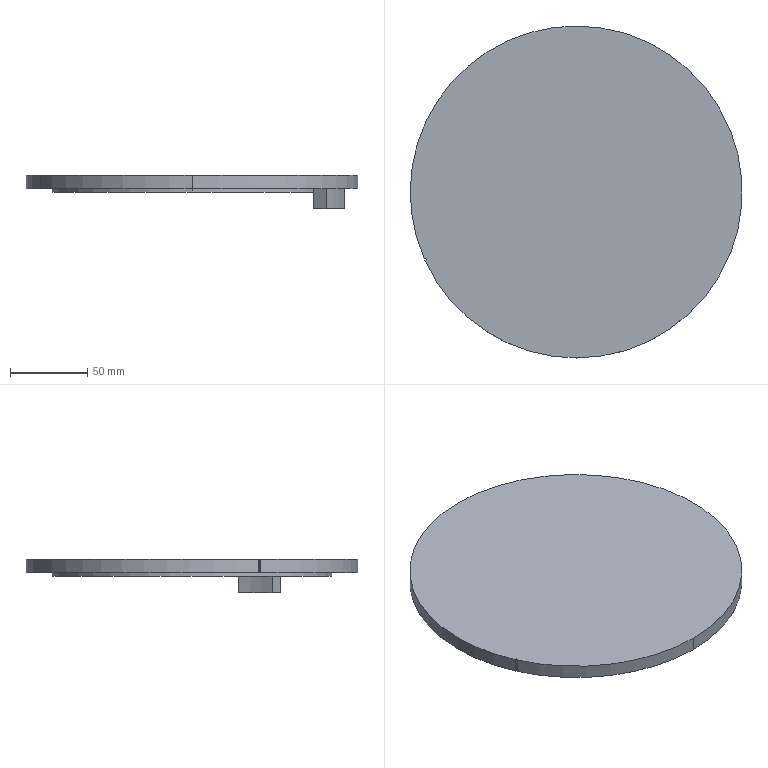Part | STEP file | ASND-0110-IRB120_3-58_IRC5_Link1_rev0-1 | 2 solids | 17 faces | box 215 x 215 x 22 mm | volume 381566 mm3 | plane 10 | cylinder 7 | commonest cylinder face diameters 215 x3 181 x2 188 x1 208 x1
STEP:
#1=CARTESIAN_POINT('',(0.,0.,0.));
#2=DIRECTION('',(0.,0.,1.));
#3=DIRECTION('',(1.,0.,0.));
#4=AXIS2_PLACEMENT_3D('',#1,#2,#3);
#5=CARTESIAN_POINT('',(86.724,-57.401,155.));
#6=VERTEX_POINT('',#5);
#7=CARTESIAN_POINT('',(98.626,-33.,155.));
#8=VERTEX_POINT('',#7);
#9=CARTESIAN_POINT('',(0.,0.,155.));
#10=DIRECTION('',(0.,0.,1.));
#11=DIRECTION('',(0.8988,-0.4384,0.));
#12=AXIS2_PLACEMENT_3D('',#9,#10,#11);
#13=CIRCLE('',#12,104.);
#14=CARTESIAN_POINT('',(0.,0.,168.));
#15=DIRECTION('',(0.,0.,-1.));
#16=DIRECTION('',(-0.8988,0.4384,0.));
#17=AXIS2_PLACEMENT_3D('',#14,#15,#16);
#18=CYLINDRICAL_SURFACE('',#17,104.);
#19=CARTESIAN_POINT('',(9.425,13.));
#20=DIRECTION('',(-1.,0.));
#21=VECTOR('',#20,1.);
#22=LINE('',#19,#21);
#23=(GEOMETRIC_REPRESENTATION_CONTEXT(2)PARAMETRIC_REPRESENTATION_CONTEXT()REPRESENTATION_CONTEXT('',''));
#24=DEFINITIONAL_REPRESENTATION('',(#22),#23);
#25=PCURVE('',#18,#24);
#26=CARTESIAN_POINT('',(0.,0.,155.));
#27=DIRECTION('',(0.,0.,1.));
#28=DIRECTION('',(0.7071,0.7071,0.));
#29=AXIS2_PLACEMENT_3D('',#26,#27,#28);
#30=PLANE('',#29);
#31=CARTESIAN_POINT('',(0.,0.));
#32=DIRECTION('',(0.3256,-0.9455));
#33=AXIS2_PLACEMENT_2D('',#31,#32);
#34=CIRCLE('',#33,104.);
#35=(GEOMETRIC_REPRESENTATION_CONTEXT(2)PARAMETRIC_REPRESENTATION_CONTEXT()REPRESENTATION_CONTEXT('',''));
#36=DEFINITIONAL_REPRESENTATION('',(#34),#35);
#37=PCURVE('',#30,#36);
#38=SURFACE_CURVE('',#13,(#25,#37),.PCURVE_S1.);
#39=EDGE_CURVE('',#6,#8,#38,.T.);
#40=ORIENTED_EDGE('',*,*,#39,.T.);
#41=CARTESIAN_POINT('',(98.626,-33.,168.));
#42=VERTEX_POINT('',#41);
#43=CARTESIAN_POINT('',(98.626,-33.,168.));
#44=DIRECTION('',(0.,0.,-1.));
#45=VECTOR('',#44,1.);
#46=LINE('',#43,#45);
#47=CARTESIAN_POINT('',(3.011,0.));
#48=DIRECTION('',(0.,1.));
#49=VECTOR('',#48,1.);
#50=LINE('',#47,#49);
#51=(GEOMETRIC_REPRESENTATION_CONTEXT(2)PARAMETRIC_REPRESENTATION_CONTEXT()REPRESENTATION_CONTEXT('',''));
#52=DEFINITIONAL_REPRESENTATION('',(#50),#51);
#53=PCURVE('',#18,#52);
#54=CARTESIAN_POINT('',(98.626,-33.,168.));
#55=DIRECTION('',(-0.3173,-0.9483,0.));
#56=DIRECTION('',(0.6881,-0.2302,0.6881));
#57=AXIS2_PLACEMENT_3D('',#54,#55,#56);
#58=PLANE('',#57);
#59=CARTESIAN_POINT('',(0.,0.));
#60=DIRECTION('',(-0.6881,-0.7256));
#61=VECTOR('',#60,1.);
#62=LINE('',#59,#61);
#63=(GEOMETRIC_REPRESENTATION_CONTEXT(2)PARAMETRIC_REPRESENTATION_CONTEXT()REPRESENTATION_CONTEXT('',''));
#64=DEFINITIONAL_REPRESENTATION('',(#62),#63);
#65=PCURVE('',#58,#64);
#66=SURFACE_CURVE('',#46,(#53,#65),.PCURVE_S1.);
#67=EDGE_CURVE('',#42,#8,#66,.T.);
#68=ORIENTED_EDGE('',*,*,#67,.F.);
#69=CARTESIAN_POINT('',(86.724,-57.401,168.));
#70=VERTEX_POINT('',#69);
#71=CARTESIAN_POINT('',(0.,0.,168.));
#72=DIRECTION('',(0.,0.,1.));
#73=DIRECTION('',(0.8988,-0.4384,0.));
#74=AXIS2_PLACEMENT_3D('',#71,#72,#73);
#75=CIRCLE('',#74,104.);
#76=CARTESIAN_POINT('',(9.425,0.));
#77=DIRECTION('',(-1.,0.));
#78=VECTOR('',#77,1.);
#79=LINE('',#76,#78);
#80=(GEOMETRIC_REPRESENTATION_CONTEXT(2)PARAMETRIC_REPRESENTATION_CONTEXT()REPRESENTATION_CONTEXT('',''));
#81=DEFINITIONAL_REPRESENTATION('',(#79),#80);
#82=PCURVE('',#18,#81);
#83=CARTESIAN_POINT('',(0.,0.,168.));
#84=DIRECTION('',(0.,0.,1.));
#85=DIRECTION('',(0.7071,0.7071,0.));
#86=AXIS2_PLACEMENT_3D('',#83,#84,#85);
#87=PLANE('',#86);
#88=CARTESIAN_POINT('',(0.,0.));
#89=DIRECTION('',(0.3256,-0.9455));
#90=AXIS2_PLACEMENT_2D('',#88,#89);
#91=CIRCLE('',#90,104.);
#92=(GEOMETRIC_REPRESENTATION_CONTEXT(2)PARAMETRIC_REPRESENTATION_CONTEXT()REPRESENTATION_CONTEXT('',''));
#93=DEFINITIONAL_REPRESENTATION('',(#91),#92);
#94=PCURVE('',#87,#93);
#95=SURFACE_CURVE('',#75,(#82,#94),.PCURVE_S1.);
#96=EDGE_CURVE('',#70,#42,#95,.T.);
#97=ORIENTED_EDGE('',*,*,#96,.F.);
#98=CARTESIAN_POINT('',(86.724,-57.401,168.));
#99=DIRECTION('',(0.,0.,-1.));
#100=VECTOR('',#99,1.);
#101=LINE('',#98,#100);
#102=CARTESIAN_POINT('',(3.272,0.));
#103=DIRECTION('',(0.,1.));
#104=VECTOR('',#103,1.);
#105=LINE('',#102,#104);
#106=(GEOMETRIC_REPRESENTATION_CONTEXT(2)PARAMETRIC_REPRESENTATION_CONTEXT()REPRESENTATION_CONTEXT('',''));
#107=DEFINITIONAL_REPRESENTATION('',(#105),#106);
#108=PCURVE('',#18,#107);
#109=CARTESIAN_POINT('',(86.724,-57.401,168.));
#110=DIRECTION('',(0.5519,0.8339,0.));
#111=DIRECTION('',(-0.7301,0.4832,0.4832));
#112=AXIS2_PLACEMENT_3D('',#109,#110,#111);
#113=PLANE('',#112);
#114=CARTESIAN_POINT('',(0.,0.));
#115=DIRECTION('',(-0.4832,-0.8755));
#116=VECTOR('',#115,1.);
#117=LINE('',#114,#116);
#118=(GEOMETRIC_REPRESENTATION_CONTEXT(2)PARAMETRIC_REPRESENTATION_CONTEXT()REPRESENTATION_CONTEXT('',''));
#119=DEFINITIONAL_REPRESENTATION('',(#117),#118);
#120=PCURVE('',#113,#119);
#121=SURFACE_CURVE('',#101,(#108,#120),.PCURVE_S1.);
#122=EDGE_CURVE('',#70,#6,#121,.T.);
#123=ORIENTED_EDGE('',*,*,#122,.T.);
#124=EDGE_LOOP('',(#40,#68,#97,#123));
#125=FACE_BOUND('',#124,.T.);
#126=ADVANCED_FACE('',(#125),#18,.T.);
#127=CARTESIAN_POINT('',(89.142,-29.827,155.));
#128=VERTEX_POINT('',#127);
#129=CARTESIAN_POINT('',(98.626,-33.,155.));
#130=DIRECTION('',(-0.9483,0.3173,0.));
#131=VECTOR('',#130,1.);
#132=LINE('',#129,#131);
#133=CARTESIAN_POINT('',(-8.945,-9.433));
#134=DIRECTION('',(-0.7256,0.6881));
#135=VECTOR('',#134,1.);
#136=LINE('',#133,#135);
#137=(GEOMETRIC_REPRESENTATION_CONTEXT(2)PARAMETRIC_REPRESENTATION_CONTEXT()REPRESENTATION_CONTEXT('',''));
#138=DEFINITIONAL_REPRESENTATION('',(#136),#137);
#139=PCURVE('',#58,#138);
#140=CARTESIAN_POINT('',(46.405,-93.073));
#141=DIRECTION('',(-0.4462,0.8949));
#142=VECTOR('',#141,1.);
#143=LINE('',#140,#142);
#144=(GEOMETRIC_REPRESENTATION_CONTEXT(2)PARAMETRIC_REPRESENTATION_CONTEXT()REPRESENTATION_CONTEXT('',''));
#145=DEFINITIONAL_REPRESENTATION('',(#143),#144);
#146=PCURVE('',#30,#145);
#147=SURFACE_CURVE('',#132,(#139,#146),.PCURVE_S1.);
#148=EDGE_CURVE('',#8,#128,#147,.T.);
#149=ORIENTED_EDGE('',*,*,#148,.T.);
#150=CARTESIAN_POINT('',(89.142,-29.827,168.));
#151=VERTEX_POINT('',#150);
#152=CARTESIAN_POINT('',(89.142,-29.827,168.));
#153=DIRECTION('',(0.,0.,-1.));
#154=VECTOR('',#153,1.);
#155=LINE('',#152,#154);
#156=CARTESIAN_POINT('',(-7.256,6.881));
#157=DIRECTION('',(-0.6881,-0.7256));
#158=VECTOR('',#157,1.);
#159=LINE('',#156,#158);
#160=(GEOMETRIC_REPRESENTATION_CONTEXT(2)PARAMETRIC_REPRESENTATION_CONTEXT()REPRESENTATION_CONTEXT('',''));
#161=DEFINITIONAL_REPRESENTATION('',(#159),#160);
#162=PCURVE('',#58,#161);
#163=CARTESIAN_POINT('',(0.,0.,168.));
#164=DIRECTION('',(0.,0.,-1.));
#165=DIRECTION('',(-0.8988,0.4384,0.));
#166=AXIS2_PLACEMENT_3D('',#163,#164,#165);
#167=CYLINDRICAL_SURFACE('',#166,94.);
#168=CARTESIAN_POINT('',(3.011,0.));
#169=DIRECTION('',(0.,1.));
#170=VECTOR('',#169,1.);
#171=LINE('',#168,#170);
#172=(GEOMETRIC_REPRESENTATION_CONTEXT(2)PARAMETRIC_REPRESENTATION_CONTEXT()REPRESENTATION_CONTEXT('',''));
#173=DEFINITIONAL_REPRESENTATION('',(#171),#172);
#174=PCURVE('',#167,#173);
#175=SURFACE_CURVE('',#155,(#162,#174),.PCURVE_S1.);
#176=EDGE_CURVE('',#151,#128,#175,.T.);
#177=ORIENTED_EDGE('',*,*,#176,.F.);
#178=CARTESIAN_POINT('',(98.626,-33.,168.));
#179=DIRECTION('',(-0.9483,0.3173,0.));
#180=VECTOR('',#179,1.);
#181=LINE('',#178,#180);
#182=CARTESIAN_POINT('',(0.,0.));
#183=DIRECTION('',(-0.7256,0.6881));
#184=VECTOR('',#183,1.);
#185=LINE('',#182,#184);
#186=(GEOMETRIC_REPRESENTATION_CONTEXT(2)PARAMETRIC_REPRESENTATION_CONTEXT()REPRESENTATION_CONTEXT('',''));
#187=DEFINITIONAL_REPRESENTATION('',(#185),#186);
#188=PCURVE('',#58,#187);
#189=CARTESIAN_POINT('',(46.405,-93.073));
#190=DIRECTION('',(-0.4462,0.8949));
#191=VECTOR('',#190,1.);
#192=LINE('',#189,#191);
#193=(GEOMETRIC_REPRESENTATION_CONTEXT(2)PARAMETRIC_REPRESENTATION_CONTEXT()REPRESENTATION_CONTEXT('',''));
#194=DEFINITIONAL_REPRESENTATION('',(#192),#193);
#195=PCURVE('',#87,#194);
#196=SURFACE_CURVE('',#181,(#188,#195),.PCURVE_S1.);
#197=EDGE_CURVE('',#42,#151,#196,.T.);
#198=ORIENTED_EDGE('',*,*,#197,.F.);
#199=ORIENTED_EDGE('',*,*,#67,.T.);
#200=EDGE_LOOP('',(#149,#177,#198,#199));
#201=FACE_BOUND('',#200,.T.);
#202=ADVANCED_FACE('',(#201),#58,.F.);
#203=ORIENTED_EDGE('',*,*,#176,.F.);
#204=CARTESIAN_POINT('',(78.385,-51.882,168.));
#205=VERTEX_POINT('',#204);
#206=CARTESIAN_POINT('',(0.,0.,168.));
#207=DIRECTION('',(0.,0.,-1.));
#208=DIRECTION('',(0.8988,-0.4384,0.));
#209=AXIS2_PLACEMENT_3D('',#206,#207,#208);
#210=CIRCLE('',#209,94.);
#211=CARTESIAN_POINT('',(-3.142,0.));
#212=DIRECTION('',(1.,0.));
#213=VECTOR('',#212,1.);
#214=LINE('',#211,#213);
#215=(GEOMETRIC_REPRESENTATION_CONTEXT(2)PARAMETRIC_REPRESENTATION_CONTEXT()REPRESENTATION_CONTEXT('',''));
#216=DEFINITIONAL_REPRESENTATION('',(#214),#215);
#217=PCURVE('',#167,#216);
#218=CARTESIAN_POINT('',(30.603,-88.879));
#219=CARTESIAN_POINT('',(-123.339,-141.885));
#220=CARTESIAN_POINT('',(-92.273,17.936));
#221=CARTESIAN_POINT('',(-61.207,177.757));
#222=CARTESIAN_POINT('',(61.67,70.943));
#223=CARTESIAN_POINT('',(184.546,-35.872));
#224=CARTESIAN_POINT('',(30.603,-88.879));
#225=(BOUNDED_CURVE()B_SPLINE_CURVE(2,(#218,#219,#220,#221,#222,#223,#224),.UNSPECIFIED.,.T.,.F.)B_SPLINE_CURVE_WITH_KNOTS((1,2,2,2,2,1),(-2.094,0.,2.094,4.189,6.283,8.378),.UNSPECIFIED.)CURVE()GEOMETRIC_REPRESENTATION_ITEM()RATIONAL_B_SPLINE_CURVE((1.,0.5,1.,0.5,1.,0.5,1.))REPRESENTATION_ITEM(''));
#226=(GEOMETRIC_REPRESENTATION_CONTEXT(2)PARAMETRIC_REPRESENTATION_CONTEXT()REPRESENTATION_CONTEXT('',''));
#227=DEFINITIONAL_REPRESENTATION('',(#225),#226);
#228=PCURVE('',#87,#227);
#229=SURFACE_CURVE('',#210,(#217,#228),.PCURVE_S1.);
#230=EDGE_CURVE('',#151,#205,#229,.T.);
#231=ORIENTED_EDGE('',*,*,#230,.T.);
#232=CARTESIAN_POINT('',(78.385,-51.882,155.));
#233=VERTEX_POINT('',#232);
#234=CARTESIAN_POINT('',(78.385,-51.882,168.));
#235=DIRECTION('',(0.,0.,-1.));
#236=VECTOR('',#235,1.);
#237=LINE('',#234,#236);
#238=CARTESIAN_POINT('',(3.272,0.));
#239=DIRECTION('',(0.,1.));
#240=VECTOR('',#239,1.);
#241=LINE('',#238,#240);
#242=(GEOMETRIC_REPRESENTATION_CONTEXT(2)PARAMETRIC_REPRESENTATION_CONTEXT()REPRESENTATION_CONTEXT('',''));
#243=DEFINITIONAL_REPRESENTATION('',(#241),#242);
#244=PCURVE('',#167,#243);
#245=CARTESIAN_POINT('',(8.755,-4.832));
#246=DIRECTION('',(-0.4832,-0.8755));
#247=VECTOR('',#246,1.);
#248=LINE('',#245,#247);
#249=(GEOMETRIC_REPRESENTATION_CONTEXT(2)PARAMETRIC_REPRESENTATION_CONTEXT()REPRESENTATION_CONTEXT('',''));
#250=DEFINITIONAL_REPRESENTATION('',(#248),#249);
#251=PCURVE('',#113,#250);
#252=SURFACE_CURVE('',#237,(#244,#251),.PCURVE_S1.);
#253=EDGE_CURVE('',#205,#233,#252,.T.);
#254=ORIENTED_EDGE('',*,*,#253,.T.);
#255=CARTESIAN_POINT('',(0.,0.,155.));
#256=DIRECTION('',(0.,0.,-1.));
#257=DIRECTION('',(0.8988,-0.4384,0.));
#258=AXIS2_PLACEMENT_3D('',#255,#256,#257);
#259=CIRCLE('',#258,94.);
#260=CARTESIAN_POINT('',(-3.142,13.));
#261=DIRECTION('',(1.,0.));
#262=VECTOR('',#261,1.);
#263=LINE('',#260,#262);
#264=(GEOMETRIC_REPRESENTATION_CONTEXT(2)PARAMETRIC_REPRESENTATION_CONTEXT()REPRESENTATION_CONTEXT('',''));
#265=DEFINITIONAL_REPRESENTATION('',(#263),#264);
#266=PCURVE('',#167,#265);
#267=CARTESIAN_POINT('',(30.603,-88.879));
#268=CARTESIAN_POINT('',(-123.339,-141.885));
#269=CARTESIAN_POINT('',(-92.273,17.936));
#270=CARTESIAN_POINT('',(-61.207,177.757));
#271=CARTESIAN_POINT('',(61.67,70.943));
#272=CARTESIAN_POINT('',(184.546,-35.872));
#273=CARTESIAN_POINT('',(30.603,-88.879));
#274=(BOUNDED_CURVE()B_SPLINE_CURVE(2,(#267,#268,#269,#270,#271,#272,#273),.UNSPECIFIED.,.T.,.F.)B_SPLINE_CURVE_WITH_KNOTS((1,2,2,2,2,1),(-2.094,0.,2.094,4.189,6.283,8.378),.UNSPECIFIED.)CURVE()GEOMETRIC_REPRESENTATION_ITEM()RATIONAL_B_SPLINE_CURVE((1.,0.5,1.,0.5,1.,0.5,1.))REPRESENTATION_ITEM(''));
#275=(GEOMETRIC_REPRESENTATION_CONTEXT(2)PARAMETRIC_REPRESENTATION_CONTEXT()REPRESENTATION_CONTEXT('',''));
#276=DEFINITIONAL_REPRESENTATION('',(#274),#275);
#277=PCURVE('',#30,#276);
#278=SURFACE_CURVE('',#259,(#266,#277),.PCURVE_S1.);
#279=EDGE_CURVE('',#128,#233,#278,.T.);
#280=ORIENTED_EDGE('',*,*,#279,.F.);
#281=EDGE_LOOP('',(#203,#231,#254,#280));
#282=FACE_BOUND('',#281,.F.);
#283=ADVANCED_FACE('',(#282),#167,.F.);
#284=CARTESIAN_POINT('',(78.385,-51.882,155.));
#285=DIRECTION('',(0.8339,-0.5519,0.));
#286=VECTOR('',#285,1.);
#287=LINE('',#284,#286);
#288=CARTESIAN_POINT('',(2.473,-16.214));
#289=DIRECTION('',(-0.8755,0.4832));
#290=VECTOR('',#289,1.);
#291=LINE('',#288,#290);
#292=(GEOMETRIC_REPRESENTATION_CONTEXT(2)PARAMETRIC_REPRESENTATION_CONTEXT()REPRESENTATION_CONTEXT('',''));
#293=DEFINITIONAL_REPRESENTATION('',(#291),#292);
#294=PCURVE('',#113,#293);
#295=CARTESIAN_POINT('',(18.741,-92.113));
#296=DIRECTION('',(0.1994,-0.9799));
#297=VECTOR('',#296,1.);
#298=LINE('',#295,#297);
#299=(GEOMETRIC_REPRESENTATION_CONTEXT(2)PARAMETRIC_REPRESENTATION_CONTEXT()REPRESENTATION_CONTEXT('',''));
#300=DEFINITIONAL_REPRESENTATION('',(#298),#299);
#301=PCURVE('',#30,#300);
#302=SURFACE_CURVE('',#287,(#294,#301),.PCURVE_S1.);
#303=EDGE_CURVE('',#233,#6,#302,.T.);
#304=ORIENTED_EDGE('',*,*,#303,.T.);
#305=ORIENTED_EDGE('',*,*,#122,.F.);
#306=CARTESIAN_POINT('',(78.385,-51.882,168.));
#307=DIRECTION('',(0.8339,-0.5519,0.));
#308=VECTOR('',#307,1.);
#309=LINE('',#306,#308);
#310=CARTESIAN_POINT('',(8.755,-4.832));
#311=DIRECTION('',(-0.8755,0.4832));
#312=VECTOR('',#311,1.);
#313=LINE('',#310,#312);
#314=(GEOMETRIC_REPRESENTATION_CONTEXT(2)PARAMETRIC_REPRESENTATION_CONTEXT()REPRESENTATION_CONTEXT('',''));
#315=DEFINITIONAL_REPRESENTATION('',(#313),#314);
#316=PCURVE('',#113,#315);
#317=CARTESIAN_POINT('',(18.741,-92.113));
#318=DIRECTION('',(0.1994,-0.9799));
#319=VECTOR('',#318,1.);
#320=LINE('',#317,#319);
#321=(GEOMETRIC_REPRESENTATION_CONTEXT(2)PARAMETRIC_REPRESENTATION_CONTEXT()REPRESENTATION_CONTEXT('',''));
#322=DEFINITIONAL_REPRESENTATION('',(#320),#321);
#323=PCURVE('',#87,#322);
#324=SURFACE_CURVE('',#309,(#316,#323),.PCURVE_S1.);
#325=EDGE_CURVE('',#205,#70,#324,.T.);
#326=ORIENTED_EDGE('',*,*,#325,.F.);
#327=ORIENTED_EDGE('',*,*,#253,.T.);
#328=EDGE_LOOP('',(#304,#305,#326,#327));
#329=FACE_BOUND('',#328,.T.);
#330=ADVANCED_FACE('',(#329),#113,.F.);
#331=ORIENTED_EDGE('',*,*,#96,.T.);
#332=ORIENTED_EDGE('',*,*,#197,.T.);
#333=ORIENTED_EDGE('',*,*,#230,.T.);
#334=ORIENTED_EDGE('',*,*,#325,.T.);
#335=EDGE_LOOP('',(#331,#332,#333,#334));
#336=FACE_BOUND('',#335,.T.);
#337=ADVANCED_FACE('',(#336),#87,.T.);
#338=ORIENTED_EDGE('',*,*,#39,.F.);
#339=ORIENTED_EDGE('',*,*,#303,.F.);
#340=ORIENTED_EDGE('',*,*,#279,.F.);
#341=ORIENTED_EDGE('',*,*,#148,.F.);
#342=EDGE_LOOP('',(#338,#339,#340,#341));
#343=FACE_BOUND('',#342,.T.);
#344=ADVANCED_FACE('',(#343),#30,.F.);
#345=CLOSED_SHELL('',(#126,#202,#283,#330,#337,#344));
#346=MANIFOLD_SOLID_BREP('',#345);
#347=CARTESIAN_POINT('',(0.,90.5,166.));
#348=VERTEX_POINT('',#347);
#349=CARTESIAN_POINT('',(0.,-90.5,166.));
#350=VERTEX_POINT('',#349);
#351=CARTESIAN_POINT('',(0.,0.,166.));
#352=DIRECTION('',(0.,0.,-1.));
#353=DIRECTION('',(0.,1.,0.));
#354=AXIS2_PLACEMENT_3D('',#351,#352,#353);
#355=CIRCLE('',#354,90.5);
#356=CARTESIAN_POINT('',(0.,0.,166.));
#357=DIRECTION('',(0.,0.,1.));
#358=DIRECTION('',(0.,-1.,0.));
#359=AXIS2_PLACEMENT_3D('',#356,#357,#358);
#360=CYLINDRICAL_SURFACE('',#359,90.5);
#361=CARTESIAN_POINT('',(3.142,0.));
#362=DIRECTION('',(-1.,0.));
#363=VECTOR('',#362,1.);
#364=LINE('',#361,#363);
#365=(GEOMETRIC_REPRESENTATION_CONTEXT(2)PARAMETRIC_REPRESENTATION_CONTEXT()REPRESENTATION_CONTEXT('',''));
#366=DEFINITIONAL_REPRESENTATION('',(#364),#365);
#367=PCURVE('',#360,#366);
#368=CARTESIAN_POINT('',(0.,0.,166.));
#369=DIRECTION('',(0.,0.,-1.));
#370=DIRECTION('',(0.7071,0.7071,0.));
#371=AXIS2_PLACEMENT_3D('',#368,#369,#370);
#372=PLANE('',#371);
#373=CARTESIAN_POINT('',(0.,0.));
#374=DIRECTION('',(0.7071,-0.7071));
#375=AXIS2_PLACEMENT_2D('',#373,#374);
#376=CIRCLE('',#375,90.5);
#377=(GEOMETRIC_REPRESENTATION_CONTEXT(2)PARAMETRIC_REPRESENTATION_CONTEXT()REPRESENTATION_CONTEXT('',''));
#378=DEFINITIONAL_REPRESENTATION('',(#376),#377);
#379=PCURVE('',#372,#378);
#380=SURFACE_CURVE('',#355,(#367,#379),.PCURVE_S1.);
#381=EDGE_CURVE('',#348,#350,#380,.T.);
#382=ORIENTED_EDGE('',*,*,#381,.F.);
#383=CARTESIAN_POINT('',(0.,90.5,168.));
#384=VERTEX_POINT('',#383);
#385=CARTESIAN_POINT('',(0.,90.5,166.));
#386=DIRECTION('',(0.,0.,1.));
#387=VECTOR('',#386,1.);
#388=LINE('',#385,#387);
#389=CARTESIAN_POINT('',(3.142,0.));
#390=DIRECTION('',(0.,1.));
#391=VECTOR('',#390,1.);
#392=LINE('',#389,#391);
#393=(GEOMETRIC_REPRESENTATION_CONTEXT(2)PARAMETRIC_REPRESENTATION_CONTEXT()REPRESENTATION_CONTEXT('',''));
#394=DEFINITIONAL_REPRESENTATION('',(#392),#393);
#395=PCURVE('',#360,#394);
#396=CARTESIAN_POINT('',(0.,0.,166.));
#397=DIRECTION('',(0.,0.,1.));
#398=DIRECTION('',(0.,-1.,0.));
#399=AXIS2_PLACEMENT_3D('',#396,#397,#398);
#400=CYLINDRICAL_SURFACE('',#399,90.5);
#401=CARTESIAN_POINT('',(3.142,0.));
#402=DIRECTION('',(0.,1.));
#403=VECTOR('',#402,1.);
#404=LINE('',#401,#403);
#405=(GEOMETRIC_REPRESENTATION_CONTEXT(2)PARAMETRIC_REPRESENTATION_CONTEXT()REPRESENTATION_CONTEXT('',''));
#406=DEFINITIONAL_REPRESENTATION('',(#404),#405);
#407=PCURVE('',#400,#406);
#408=SURFACE_CURVE('',#388,(#395,#407),.PCURVE_S1.);
#409=EDGE_CURVE('',#348,#384,#408,.T.);
#410=ORIENTED_EDGE('',*,*,#409,.T.);
#411=CARTESIAN_POINT('',(0.,-90.5,168.));
#412=VERTEX_POINT('',#411);
#413=CARTESIAN_POINT('',(0.,0.,168.));
#414=DIRECTION('',(0.,0.,-1.));
#415=DIRECTION('',(0.,1.,0.));
#416=AXIS2_PLACEMENT_3D('',#413,#414,#415);
#417=CIRCLE('',#416,90.5);
#418=CARTESIAN_POINT('',(3.142,2.));
#419=DIRECTION('',(-1.,0.));
#420=VECTOR('',#419,1.);
#421=LINE('',#418,#420);
#422=(GEOMETRIC_REPRESENTATION_CONTEXT(2)PARAMETRIC_REPRESENTATION_CONTEXT()REPRESENTATION_CONTEXT('',''));
#423=DEFINITIONAL_REPRESENTATION('',(#421),#422);
#424=PCURVE('',#360,#423);
#425=CARTESIAN_POINT('',(0.,0.,168.));
#426=DIRECTION('',(0.,0.,-1.));
#427=DIRECTION('',(0.7071,0.7071,0.));
#428=AXIS2_PLACEMENT_3D('',#425,#426,#427);
#429=PLANE('',#428);
#430=CARTESIAN_POINT('',(0.,0.));
#431=DIRECTION('',(0.7071,-0.7071));
#432=AXIS2_PLACEMENT_2D('',#430,#431);
#433=CIRCLE('',#432,90.5);
#434=(GEOMETRIC_REPRESENTATION_CONTEXT(2)PARAMETRIC_REPRESENTATION_CONTEXT()REPRESENTATION_CONTEXT('',''));
#435=DEFINITIONAL_REPRESENTATION('',(#433),#434);
#436=PCURVE('',#429,#435);
#437=SURFACE_CURVE('',#417,(#424,#436),.PCURVE_S1.);
#438=EDGE_CURVE('',#384,#412,#437,.T.);
#439=ORIENTED_EDGE('',*,*,#438,.T.);
#440=CARTESIAN_POINT('',(0.,-90.5,166.));
#441=DIRECTION('',(0.,0.,1.));
#442=VECTOR('',#441,1.);
#443=LINE('',#440,#442);
#444=CARTESIAN_POINT('',(0.,0.));
#445=DIRECTION('',(0.,1.));
#446=VECTOR('',#445,1.);
#447=LINE('',#444,#446);
#448=(GEOMETRIC_REPRESENTATION_CONTEXT(2)PARAMETRIC_REPRESENTATION_CONTEXT()REPRESENTATION_CONTEXT('',''));
#449=DEFINITIONAL_REPRESENTATION('',(#447),#448);
#450=PCURVE('',#360,#449);
#451=CARTESIAN_POINT('',(6.283,0.));
#452=DIRECTION('',(0.,1.));
#453=VECTOR('',#452,1.);
#454=LINE('',#451,#453);
#455=(GEOMETRIC_REPRESENTATION_CONTEXT(2)PARAMETRIC_REPRESENTATION_CONTEXT()REPRESENTATION_CONTEXT('',''));
#456=DEFINITIONAL_REPRESENTATION('',(#454),#455);
#457=PCURVE('',#400,#456);
#458=SURFACE_CURVE('',#443,(#450,#457),.PCURVE_S1.);
#459=EDGE_CURVE('',#350,#412,#458,.T.);
#460=ORIENTED_EDGE('',*,*,#459,.F.);
#461=EDGE_LOOP('',(#382,#410,#439,#460));
#462=FACE_BOUND('',#461,.T.);
#463=ADVANCED_FACE('',(#462),#360,.T.);
#464=CARTESIAN_POINT('',(0.,107.5,168.));
#465=VERTEX_POINT('',#464);
#466=CARTESIAN_POINT('',(0.,-107.5,168.));
#467=VERTEX_POINT('',#466);
#468=CARTESIAN_POINT('',(0.,0.,168.));
#469=DIRECTION('',(0.,0.,-1.));
#470=DIRECTION('',(0.,1.,0.));
#471=AXIS2_PLACEMENT_3D('',#468,#469,#470);
#472=CIRCLE('',#471,107.5);
#473=CARTESIAN_POINT('',(0.,0.,164.));
#474=DIRECTION('',(0.,0.,1.));
#475=DIRECTION('',(0.,-1.,0.));
#476=AXIS2_PLACEMENT_3D('',#473,#474,#475);
#477=CYLINDRICAL_SURFACE('',#476,107.5);
#478=CARTESIAN_POINT('',(3.142,4.));
#479=DIRECTION('',(-1.,0.));
#480=VECTOR('',#479,1.);
#481=LINE('',#478,#480);
#482=(GEOMETRIC_REPRESENTATION_CONTEXT(2)PARAMETRIC_REPRESENTATION_CONTEXT()REPRESENTATION_CONTEXT('',''));
#483=DEFINITIONAL_REPRESENTATION('',(#481),#482);
#484=PCURVE('',#477,#483);
#485=CARTESIAN_POINT('',(0.,0.));
#486=DIRECTION('',(0.7071,-0.7071));
#487=AXIS2_PLACEMENT_2D('',#485,#486);
#488=CIRCLE('',#487,107.5);
#489=(GEOMETRIC_REPRESENTATION_CONTEXT(2)PARAMETRIC_REPRESENTATION_CONTEXT()REPRESENTATION_CONTEXT('',''));
#490=DEFINITIONAL_REPRESENTATION('',(#488),#489);
#491=PCURVE('',#429,#490);
#492=SURFACE_CURVE('',#472,(#484,#491),.PCURVE_S1.);
#493=EDGE_CURVE('',#465,#467,#492,.T.);
#494=ORIENTED_EDGE('',*,*,#493,.F.);
#495=CARTESIAN_POINT('',(0.,107.5,177.));
#496=VERTEX_POINT('',#495);
#497=CARTESIAN_POINT('',(0.,107.5,164.));
#498=DIRECTION('',(0.,0.,1.));
#499=VECTOR('',#498,1.);
#500=LINE('',#497,#499);
#501=CARTESIAN_POINT('',(3.142,0.));
#502=DIRECTION('',(0.,1.));
#503=VECTOR('',#502,1.);
#504=LINE('',#501,#503);
#505=(GEOMETRIC_REPRESENTATION_CONTEXT(2)PARAMETRIC_REPRESENTATION_CONTEXT()REPRESENTATION_CONTEXT('',''));
#506=DEFINITIONAL_REPRESENTATION('',(#504),#505);
#507=PCURVE('',#477,#506);
#508=CARTESIAN_POINT('',(0.,0.,164.));
#509=DIRECTION('',(0.,0.,1.));
#510=DIRECTION('',(0.,-1.,0.));
#511=AXIS2_PLACEMENT_3D('',#508,#509,#510);
#512=CYLINDRICAL_SURFACE('',#511,107.5);
#513=CARTESIAN_POINT('',(3.142,0.));
#514=DIRECTION('',(0.,1.));
#515=VECTOR('',#514,1.);
#516=LINE('',#513,#515);
#517=(GEOMETRIC_REPRESENTATION_CONTEXT(2)PARAMETRIC_REPRESENTATION_CONTEXT()REPRESENTATION_CONTEXT('',''));
#518=DEFINITIONAL_REPRESENTATION('',(#516),#517);
#519=PCURVE('',#512,#518);
#520=SURFACE_CURVE('',#500,(#507,#519),.PCURVE_S1.);
#521=EDGE_CURVE('',#465,#496,#520,.T.);
#522=ORIENTED_EDGE('',*,*,#521,.T.);
#523=CARTESIAN_POINT('',(0.,-107.5,177.));
#524=VERTEX_POINT('',#523);
#525=CARTESIAN_POINT('',(0.,0.,177.));
#526=DIRECTION('',(0.,0.,1.));
#527=DIRECTION('',(0.,-1.,0.));
#528=AXIS2_PLACEMENT_3D('',#525,#526,#527);
#529=CIRCLE('',#528,107.5);
#530=CARTESIAN_POINT('',(0.,13.));
#531=DIRECTION('',(1.,0.));
#532=VECTOR('',#531,1.);
#533=LINE('',#530,#532);
#534=(GEOMETRIC_REPRESENTATION_CONTEXT(2)PARAMETRIC_REPRESENTATION_CONTEXT()REPRESENTATION_CONTEXT('',''));
#535=DEFINITIONAL_REPRESENTATION('',(#533),#534);
#536=PCURVE('',#477,#535);
#537=CARTESIAN_POINT('',(0.,0.,177.));
#538=DIRECTION('',(0.,0.,1.));
#539=DIRECTION('',(0.7071,0.7071,0.));
#540=AXIS2_PLACEMENT_3D('',#537,#538,#539);
#541=PLANE('',#540);
#542=CARTESIAN_POINT('',(0.,0.));
#543=DIRECTION('',(-0.7071,-0.7071));
#544=AXIS2_PLACEMENT_2D('',#542,#543);
#545=CIRCLE('',#544,107.5);
#546=(GEOMETRIC_REPRESENTATION_CONTEXT(2)PARAMETRIC_REPRESENTATION_CONTEXT()REPRESENTATION_CONTEXT('',''));
#547=DEFINITIONAL_REPRESENTATION('',(#545),#546);
#548=PCURVE('',#541,#547);
#549=SURFACE_CURVE('',#529,(#536,#548),.PCURVE_S1.);
#550=EDGE_CURVE('',#524,#496,#549,.T.);
#551=ORIENTED_EDGE('',*,*,#550,.F.);
#552=CARTESIAN_POINT('',(0.,-107.5,164.));
#553=DIRECTION('',(0.,0.,1.));
#554=VECTOR('',#553,1.);
#555=LINE('',#552,#554);
#556=CARTESIAN_POINT('',(0.,0.));
#557=DIRECTION('',(0.,1.));
#558=VECTOR('',#557,1.);
#559=LINE('',#556,#558);
#560=(GEOMETRIC_REPRESENTATION_CONTEXT(2)PARAMETRIC_REPRESENTATION_CONTEXT()REPRESENTATION_CONTEXT('',''));
#561=DEFINITIONAL_REPRESENTATION('',(#559),#560);
#562=PCURVE('',#477,#561);
#563=CARTESIAN_POINT('',(0.,0.,164.));
#564=DIRECTION('',(0.,0.,1.));
#565=DIRECTION('',(0.,-1.,0.));
#566=AXIS2_PLACEMENT_3D('',#563,#564,#565);
#567=CYLINDRICAL_SURFACE('',#566,107.5);
#568=CARTESIAN_POINT('',(6.283,0.));
#569=DIRECTION('',(0.,1.));
#570=VECTOR('',#569,1.);
#571=LINE('',#568,#570);
#572=(GEOMETRIC_REPRESENTATION_CONTEXT(2)PARAMETRIC_REPRESENTATION_CONTEXT()REPRESENTATION_CONTEXT('',''));
#573=DEFINITIONAL_REPRESENTATION('',(#571),#572);
#574=PCURVE('',#567,#573);
#575=SURFACE_CURVE('',#555,(#562,#574),.PCURVE_S1.);
#576=EDGE_CURVE('',#467,#524,#575,.T.);
#577=ORIENTED_EDGE('',*,*,#576,.F.);
#578=EDGE_LOOP('',(#494,#522,#551,#577));
#579=FACE_BOUND('',#578,.T.);
#580=ADVANCED_FACE('',(#579),#477,.T.);
#581=CARTESIAN_POINT('',(-98.002,-44.18,168.));
#582=VERTEX_POINT('',#581);
#583=CARTESIAN_POINT('',(0.,0.,168.));
#584=DIRECTION('',(0.,0.,-1.));
#585=DIRECTION('',(0.,1.,0.));
#586=AXIS2_PLACEMENT_3D('',#583,#584,#585);
#587=CIRCLE('',#586,107.5);
#588=CARTESIAN_POINT('',(9.425,4.));
#589=DIRECTION('',(-1.,0.));
#590=VECTOR('',#589,1.);
#591=LINE('',#588,#590);
#592=(GEOMETRIC_REPRESENTATION_CONTEXT(2)PARAMETRIC_REPRESENTATION_CONTEXT()REPRESENTATION_CONTEXT('',''));
#593=DEFINITIONAL_REPRESENTATION('',(#591),#592);
#594=PCURVE('',#567,#593);
#595=CARTESIAN_POINT('',(0.,0.));
#596=DIRECTION('',(0.7071,-0.7071));
#597=AXIS2_PLACEMENT_2D('',#595,#596);
#598=CIRCLE('',#597,107.5);
#599=(GEOMETRIC_REPRESENTATION_CONTEXT(2)PARAMETRIC_REPRESENTATION_CONTEXT()REPRESENTATION_CONTEXT('',''));
#600=DEFINITIONAL_REPRESENTATION('',(#598),#599);
#601=PCURVE('',#429,#600);
#602=SURFACE_CURVE('',#587,(#594,#601),.PCURVE_S1.);
#603=EDGE_CURVE('',#467,#582,#602,.T.);
#604=ORIENTED_EDGE('',*,*,#603,.F.);
#605=ORIENTED_EDGE('',*,*,#576,.T.);
#606=CARTESIAN_POINT('',(-98.002,-44.18,177.));
#607=VERTEX_POINT('',#606);
#608=CARTESIAN_POINT('',(0.,0.,177.));
#609=DIRECTION('',(0.,0.,1.));
#610=DIRECTION('',(0.,-1.,0.));
#611=AXIS2_PLACEMENT_3D('',#608,#609,#610);
#612=CIRCLE('',#611,107.5);
#613=CARTESIAN_POINT('',(0.,13.));
#614=DIRECTION('',(1.,0.));
#615=VECTOR('',#614,1.);
#616=LINE('',#613,#615);
#617=(GEOMETRIC_REPRESENTATION_CONTEXT(2)PARAMETRIC_REPRESENTATION_CONTEXT()REPRESENTATION_CONTEXT('',''));
#618=DEFINITIONAL_REPRESENTATION('',(#616),#617);
#619=PCURVE('',#567,#618);
#620=CARTESIAN_POINT('',(0.,0.));
#621=DIRECTION('',(-0.7071,-0.7071));
#622=AXIS2_PLACEMENT_2D('',#620,#621);
#623=CIRCLE('',#622,107.5);
#624=(GEOMETRIC_REPRESENTATION_CONTEXT(2)PARAMETRIC_REPRESENTATION_CONTEXT()REPRESENTATION_CONTEXT('',''));
#625=DEFINITIONAL_REPRESENTATION('',(#623),#624);
#626=PCURVE('',#541,#625);
#627=SURFACE_CURVE('',#612,(#619,#626),.PCURVE_S1.);
#628=EDGE_CURVE('',#607,#524,#627,.T.);
#629=ORIENTED_EDGE('',*,*,#628,.F.);
#630=CARTESIAN_POINT('',(-98.002,-44.18,177.));
#631=DIRECTION('',(0.,0.,-1.));
#632=VECTOR('',#631,1.);
#633=LINE('',#630,#632);
#634=CARTESIAN_POINT('',(5.136,13.));
#635=DIRECTION('',(0.,-1.));
#636=VECTOR('',#635,1.);
#637=LINE('',#634,#636);
#638=(GEOMETRIC_REPRESENTATION_CONTEXT(2)PARAMETRIC_REPRESENTATION_CONTEXT()REPRESENTATION_CONTEXT('',''));
#639=DEFINITIONAL_REPRESENTATION('',(#637),#638);
#640=PCURVE('',#567,#639);
#641=CARTESIAN_POINT('',(-98.002,-44.18,181.001));
#642=DIRECTION('',(0.4067,-0.9135,0.));
#643=DIRECTION('',(0.6745,0.3003,0.6745));
#644=AXIS2_PLACEMENT_3D('',#641,#642,#643);
#645=PLANE('',#644);
#646=CARTESIAN_POINT('',(-2.699,-2.954));
#647=DIRECTION('',(-0.6745,-0.7383));
#648=VECTOR('',#647,1.);
#649=LINE('',#646,#648);
#650=(GEOMETRIC_REPRESENTATION_CONTEXT(2)PARAMETRIC_REPRESENTATION_CONTEXT()REPRESENTATION_CONTEXT('',''));
#651=DEFINITIONAL_REPRESENTATION('',(#649),#650);
#652=PCURVE('',#645,#651);
#653=SURFACE_CURVE('',#633,(#640,#652),.PCURVE_S1.);
#654=EDGE_CURVE('',#607,#582,#653,.T.);
#655=ORIENTED_EDGE('',*,*,#654,.T.);
#656=EDGE_LOOP('',(#604,#605,#629,#655));
#657=FACE_BOUND('',#656,.T.);
#658=ADVANCED_FACE('',(#657),#567,.T.);
#659=CARTESIAN_POINT('',(-97.088,-43.774,168.));
#660=VERTEX_POINT('',#659);
#661=CARTESIAN_POINT('',(-98.002,-44.18,168.));
#662=DIRECTION('',(0.9135,0.4067,0.));
#663=VECTOR('',#662,1.);
#664=LINE('',#661,#663);
#665=CARTESIAN_POINT('',(-100.538,-38.057));
#666=DIRECTION('',(0.9336,0.3584));
#667=VECTOR('',#666,1.);
#668=LINE('',#665,#667);
#669=(GEOMETRIC_REPRESENTATION_CONTEXT(2)PARAMETRIC_REPRESENTATION_CONTEXT()REPRESENTATION_CONTEXT('',''));
#670=DEFINITIONAL_REPRESENTATION('',(#668),#669);
#671=PCURVE('',#429,#670);
#672=CARTESIAN_POINT('',(-8.769,-9.599));
#673=DIRECTION('',(0.7383,-0.6745));
#674=VECTOR('',#673,1.);
#675=LINE('',#672,#674);
#676=(GEOMETRIC_REPRESENTATION_CONTEXT(2)PARAMETRIC_REPRESENTATION_CONTEXT()REPRESENTATION_CONTEXT('',''));
#677=DEFINITIONAL_REPRESENTATION('',(#675),#676);
#678=PCURVE('',#645,#677);
#679=SURFACE_CURVE('',#664,(#671,#678),.PCURVE_S1.);
#680=EDGE_CURVE('',#582,#660,#679,.T.);
#681=ORIENTED_EDGE('',*,*,#680,.T.);
#682=CARTESIAN_POINT('',(-97.495,-42.86,168.));
#683=VERTEX_POINT('',#682);
#684=CARTESIAN_POINT('',(-97.088,-43.774,168.));
#685=DIRECTION('',(-0.4067,0.9135,0.));
#686=VECTOR('',#685,1.);
#687=LINE('',#684,#686);
#688=CARTESIAN_POINT('',(-99.604,-37.699));
#689=DIRECTION('',(0.3584,-0.9336));
#690=VECTOR('',#689,1.);
#691=LINE('',#688,#690);
#692=(GEOMETRIC_REPRESENTATION_CONTEXT(2)PARAMETRIC_REPRESENTATION_CONTEXT()REPRESENTATION_CONTEXT('',''));
#693=DEFINITIONAL_REPRESENTATION('',(#691),#692);
#694=PCURVE('',#429,#693);
#695=CARTESIAN_POINT('',(-97.088,-43.774,181.001));
#696=DIRECTION('',(0.9135,0.4067,0.));
#697=DIRECTION('',(-0.3003,0.6745,0.6745));
#698=AXIS2_PLACEMENT_3D('',#695,#696,#697);
#699=PLANE('',#698);
#700=CARTESIAN_POINT('',(-8.769,-9.599));
#701=DIRECTION('',(0.7383,-0.6745));
#702=VECTOR('',#701,1.);
#703=LINE('',#700,#702);
#704=(GEOMETRIC_REPRESENTATION_CONTEXT(2)PARAMETRIC_REPRESENTATION_CONTEXT()REPRESENTATION_CONTEXT('',''));
#705=DEFINITIONAL_REPRESENTATION('',(#703),#704);
#706=PCURVE('',#699,#705);
#707=SURFACE_CURVE('',#687,(#694,#706),.PCURVE_S1.);
#708=EDGE_CURVE('',#660,#683,#707,.T.);
#709=ORIENTED_EDGE('',*,*,#708,.T.);
#710=CARTESIAN_POINT('',(-98.408,-43.267,168.));
#711=VERTEX_POINT('',#710);
#712=CARTESIAN_POINT('',(-97.495,-42.86,168.));
#713=DIRECTION('',(-0.9135,-0.4067,0.));
#714=VECTOR('',#713,1.);
#715=LINE('',#712,#714);
#716=CARTESIAN_POINT('',(-99.246,-38.633));
#717=DIRECTION('',(-0.9336,-0.3584));
#718=VECTOR('',#717,1.);
#719=LINE('',#716,#718);
#720=(GEOMETRIC_REPRESENTATION_CONTEXT(2)PARAMETRIC_REPRESENTATION_CONTEXT()REPRESENTATION_CONTEXT('',''));
#721=DEFINITIONAL_REPRESENTATION('',(#719),#720);
#722=PCURVE('',#429,#721);
#723=CARTESIAN_POINT('',(-97.495,-42.86,181.001));
#724=DIRECTION('',(-0.4067,0.9135,0.));
#725=DIRECTION('',(0.6745,0.3003,0.6745));
#726=AXIS2_PLACEMENT_3D('',#723,#724,#725);
#727=PLANE('',#726);
#728=CARTESIAN_POINT('',(-8.769,9.599));
#729=DIRECTION('',(-0.7383,-0.6745));
#730=VECTOR('',#729,1.);
#731=LINE('',#728,#730);
#732=(GEOMETRIC_REPRESENTATION_CONTEXT(2)PARAMETRIC_REPRESENTATION_CONTEXT()REPRESENTATION_CONTEXT('',''));
#733=DEFINITIONAL_REPRESENTATION('',(#731),#732);
#734=PCURVE('',#727,#733);
#735=SURFACE_CURVE('',#715,(#722,#734),.PCURVE_S1.);
#736=EDGE_CURVE('',#683,#711,#735,.T.);
#737=ORIENTED_EDGE('',*,*,#736,.T.);
#738=CARTESIAN_POINT('',(0.,0.,168.));
#739=DIRECTION('',(0.,0.,-1.));
#740=DIRECTION('',(0.,1.,0.));
#741=AXIS2_PLACEMENT_3D('',#738,#739,#740);
#742=CIRCLE('',#741,107.5);
#743=CARTESIAN_POINT('',(0.,0.));
#744=DIRECTION('',(0.7071,-0.7071));
#745=AXIS2_PLACEMENT_2D('',#743,#744);
#746=CIRCLE('',#745,107.5);
#747=(GEOMETRIC_REPRESENTATION_CONTEXT(2)PARAMETRIC_REPRESENTATION_CONTEXT()REPRESENTATION_CONTEXT('',''));
#748=DEFINITIONAL_REPRESENTATION('',(#746),#747);
#749=PCURVE('',#429,#748);
#750=CARTESIAN_POINT('',(9.425,4.));
#751=DIRECTION('',(-1.,0.));
#752=VECTOR('',#751,1.);
#753=LINE('',#750,#752);
#754=(GEOMETRIC_REPRESENTATION_CONTEXT(2)PARAMETRIC_REPRESENTATION_CONTEXT()REPRESENTATION_CONTEXT('',''));
#755=DEFINITIONAL_REPRESENTATION('',(#753),#754);
#756=PCURVE('',#512,#755);
#757=SURFACE_CURVE('',#742,(#749,#756),.PCURVE_S1.);
#758=EDGE_CURVE('',#711,#465,#757,.T.);
#759=ORIENTED_EDGE('',*,*,#758,.T.);
#760=ORIENTED_EDGE('',*,*,#493,.T.);
#761=ORIENTED_EDGE('',*,*,#603,.T.);
#762=EDGE_LOOP('',(#681,#709,#737,#759,#760,#761));
#763=FACE_BOUND('',#762,.T.);
#764=CARTESIAN_POINT('',(0.,0.,168.));
#765=DIRECTION('',(0.,0.,-1.));
#766=DIRECTION('',(0.,1.,0.));
#767=AXIS2_PLACEMENT_3D('',#764,#765,#766);
#768=CIRCLE('',#767,90.5);
#769=CARTESIAN_POINT('',(0.,0.));
#770=DIRECTION('',(0.7071,-0.7071));
#771=AXIS2_PLACEMENT_2D('',#769,#770);
#772=CIRCLE('',#771,90.5);
#773=(GEOMETRIC_REPRESENTATION_CONTEXT(2)PARAMETRIC_REPRESENTATION_CONTEXT()REPRESENTATION_CONTEXT('',''));
#774=DEFINITIONAL_REPRESENTATION('',(#772),#773);
#775=PCURVE('',#429,#774);
#776=CARTESIAN_POINT('',(9.425,2.));
#777=DIRECTION('',(-1.,0.));
#778=VECTOR('',#777,1.);
#779=LINE('',#776,#778);
#780=(GEOMETRIC_REPRESENTATION_CONTEXT(2)PARAMETRIC_REPRESENTATION_CONTEXT()REPRESENTATION_CONTEXT('',''));
#781=DEFINITIONAL_REPRESENTATION('',(#779),#780);
#782=PCURVE('',#400,#781);
#783=SURFACE_CURVE('',#768,(#775,#782),.PCURVE_S1.);
#784=EDGE_CURVE('',#412,#384,#783,.T.);
#785=ORIENTED_EDGE('',*,*,#784,.F.);
#786=ORIENTED_EDGE('',*,*,#438,.F.);
#787=EDGE_LOOP('',(#785,#786));
#788=FACE_BOUND('',#787,.T.);
#789=ADVANCED_FACE('',(#763,#788),#429,.T.);
#790=ORIENTED_EDGE('',*,*,#521,.F.);
#791=ORIENTED_EDGE('',*,*,#758,.F.);
#792=CARTESIAN_POINT('',(-98.408,-43.267,177.));
#793=VERTEX_POINT('',#792);
#794=CARTESIAN_POINT('',(-98.408,-43.267,177.));
#795=DIRECTION('',(0.,0.,-1.));
#796=VECTOR('',#795,1.);
#797=LINE('',#794,#796);
#798=CARTESIAN_POINT('',(5.127,13.));
#799=DIRECTION('',(0.,-1.));
#800=VECTOR('',#799,1.);
#801=LINE('',#798,#800);
#802=(GEOMETRIC_REPRESENTATION_CONTEXT(2)PARAMETRIC_REPRESENTATION_CONTEXT()REPRESENTATION_CONTEXT('',''));
#803=DEFINITIONAL_REPRESENTATION('',(#801),#802);
#804=PCURVE('',#512,#803);
#805=CARTESIAN_POINT('',(-3.437,2.279));
#806=DIRECTION('',(-0.6745,0.7383));
#807=VECTOR('',#806,1.);
#808=LINE('',#805,#807);
#809=(GEOMETRIC_REPRESENTATION_CONTEXT(2)PARAMETRIC_REPRESENTATION_CONTEXT()REPRESENTATION_CONTEXT('',''));
#810=DEFINITIONAL_REPRESENTATION('',(#808),#809);
#811=PCURVE('',#727,#810);
#812=SURFACE_CURVE('',#797,(#804,#811),.PCURVE_S1.);
#813=EDGE_CURVE('',#793,#711,#812,.T.);
#814=ORIENTED_EDGE('',*,*,#813,.F.);
#815=CARTESIAN_POINT('',(0.,0.,177.));
#816=DIRECTION('',(0.,0.,1.));
#817=DIRECTION('',(0.,-1.,0.));
#818=AXIS2_PLACEMENT_3D('',#815,#816,#817);
#819=CIRCLE('',#818,107.5);
#820=CARTESIAN_POINT('',(0.,13.));
#821=DIRECTION('',(1.,0.));
#822=VECTOR('',#821,1.);
#823=LINE('',#820,#822);
#824=(GEOMETRIC_REPRESENTATION_CONTEXT(2)PARAMETRIC_REPRESENTATION_CONTEXT()REPRESENTATION_CONTEXT('',''));
#825=DEFINITIONAL_REPRESENTATION('',(#823),#824);
#826=PCURVE('',#512,#825);
#827=CARTESIAN_POINT('',(0.,0.));
#828=DIRECTION('',(-0.7071,-0.7071));
#829=AXIS2_PLACEMENT_2D('',#827,#828);
#830=CIRCLE('',#829,107.5);
#831=(GEOMETRIC_REPRESENTATION_CONTEXT(2)PARAMETRIC_REPRESENTATION_CONTEXT()REPRESENTATION_CONTEXT('',''));
#832=DEFINITIONAL_REPRESENTATION('',(#830),#831);
#833=PCURVE('',#541,#832);
#834=SURFACE_CURVE('',#819,(#826,#833),.PCURVE_S1.);
#835=EDGE_CURVE('',#496,#793,#834,.T.);
#836=ORIENTED_EDGE('',*,*,#835,.F.);
#837=EDGE_LOOP('',(#790,#791,#814,#836));
#838=FACE_BOUND('',#837,.T.);
#839=ADVANCED_FACE('',(#838),#512,.T.);
#840=ORIENTED_EDGE('',*,*,#680,.F.);
#841=ORIENTED_EDGE('',*,*,#654,.F.);
#842=CARTESIAN_POINT('',(-97.088,-43.774,177.));
#843=VERTEX_POINT('',#842);
#844=CARTESIAN_POINT('',(-97.088,-43.774,177.));
#845=DIRECTION('',(-0.9135,-0.4067,0.));
#846=VECTOR('',#845,1.);
#847=LINE('',#844,#846);
#848=CARTESIAN_POINT('',(-1.96,-3.628));
#849=DIRECTION('',(-0.7383,0.6745));
#850=VECTOR('',#849,1.);
#851=LINE('',#848,#850);
#852=(GEOMETRIC_REPRESENTATION_CONTEXT(2)PARAMETRIC_REPRESENTATION_CONTEXT()REPRESENTATION_CONTEXT('',''));
#853=DEFINITIONAL_REPRESENTATION('',(#851),#852);
#854=PCURVE('',#645,#853);
#855=CARTESIAN_POINT('',(-99.604,37.699));
#856=DIRECTION('',(-0.9336,0.3584));
#857=VECTOR('',#856,1.);
#858=LINE('',#855,#857);
#859=(GEOMETRIC_REPRESENTATION_CONTEXT(2)PARAMETRIC_REPRESENTATION_CONTEXT()REPRESENTATION_CONTEXT('',''));
#860=DEFINITIONAL_REPRESENTATION('',(#858),#859);
#861=PCURVE('',#541,#860);
#862=SURFACE_CURVE('',#847,(#854,#861),.PCURVE_S1.);
#863=EDGE_CURVE('',#843,#607,#862,.T.);
#864=ORIENTED_EDGE('',*,*,#863,.F.);
#865=CARTESIAN_POINT('',(-97.088,-43.774,177.));
#866=DIRECTION('',(0.,0.,-1.));
#867=VECTOR('',#866,1.);
#868=LINE('',#865,#867);
#869=CARTESIAN_POINT('',(-1.96,-3.628));
#870=DIRECTION('',(-0.6745,-0.7383));
#871=VECTOR('',#870,1.);
#872=LINE('',#869,#871);
#873=(GEOMETRIC_REPRESENTATION_CONTEXT(2)PARAMETRIC_REPRESENTATION_CONTEXT()REPRESENTATION_CONTEXT('',''));
#874=DEFINITIONAL_REPRESENTATION('',(#872),#873);
#875=PCURVE('',#645,#874);
#876=CARTESIAN_POINT('',(-2.699,-2.954));
#877=DIRECTION('',(-0.6745,-0.7383));
#878=VECTOR('',#877,1.);
#879=LINE('',#876,#878);
#880=(GEOMETRIC_REPRESENTATION_CONTEXT(2)PARAMETRIC_REPRESENTATION_CONTEXT()REPRESENTATION_CONTEXT('',''));
#881=DEFINITIONAL_REPRESENTATION('',(#879),#880);
#882=PCURVE('',#699,#881);
#883=SURFACE_CURVE('',#868,(#875,#882),.PCURVE_S1.);
#884=EDGE_CURVE('',#843,#660,#883,.T.);
#885=ORIENTED_EDGE('',*,*,#884,.T.);
#886=EDGE_LOOP('',(#840,#841,#864,#885));
#887=FACE_BOUND('',#886,.T.);
#888=ADVANCED_FACE('',(#887),#645,.F.);
#889=ORIENTED_EDGE('',*,*,#708,.F.);
#890=ORIENTED_EDGE('',*,*,#884,.F.);
#891=CARTESIAN_POINT('',(-97.495,-42.86,177.));
#892=VERTEX_POINT('',#891);
#893=CARTESIAN_POINT('',(-97.495,-42.86,177.));
#894=DIRECTION('',(0.4067,-0.9135,0.));
#895=VECTOR('',#894,1.);
#896=LINE('',#893,#895);
#897=CARTESIAN_POINT('',(-1.96,-3.628));
#898=DIRECTION('',(-0.7383,0.6745));
#899=VECTOR('',#898,1.);
#900=LINE('',#897,#899);
#901=(GEOMETRIC_REPRESENTATION_CONTEXT(2)PARAMETRIC_REPRESENTATION_CONTEXT()REPRESENTATION_CONTEXT('',''));
#902=DEFINITIONAL_REPRESENTATION('',(#900),#901);
#903=PCURVE('',#699,#902);
#904=CARTESIAN_POINT('',(-99.246,38.633));
#905=DIRECTION('',(-0.3584,-0.9336));
#906=VECTOR('',#905,1.);
#907=LINE('',#904,#906);
#908=(GEOMETRIC_REPRESENTATION_CONTEXT(2)PARAMETRIC_REPRESENTATION_CONTEXT()REPRESENTATION_CONTEXT('',''));
#909=DEFINITIONAL_REPRESENTATION('',(#907),#908);
#910=PCURVE('',#541,#909);
#911=SURFACE_CURVE('',#896,(#903,#910),.PCURVE_S1.);
#912=EDGE_CURVE('',#892,#843,#911,.T.);
#913=ORIENTED_EDGE('',*,*,#912,.F.);
#914=CARTESIAN_POINT('',(-97.495,-42.86,177.));
#915=DIRECTION('',(0.,0.,-1.));
#916=VECTOR('',#915,1.);
#917=LINE('',#914,#916);
#918=CARTESIAN_POINT('',(-1.96,-3.628));
#919=DIRECTION('',(-0.6745,-0.7383));
#920=VECTOR('',#919,1.);
#921=LINE('',#918,#920);
#922=(GEOMETRIC_REPRESENTATION_CONTEXT(2)PARAMETRIC_REPRESENTATION_CONTEXT()REPRESENTATION_CONTEXT('',''));
#923=DEFINITIONAL_REPRESENTATION('',(#921),#922);
#924=PCURVE('',#699,#923);
#925=CARTESIAN_POINT('',(-2.699,2.954));
#926=DIRECTION('',(-0.6745,0.7383));
#927=VECTOR('',#926,1.);
#928=LINE('',#925,#927);
#929=(GEOMETRIC_REPRESENTATION_CONTEXT(2)PARAMETRIC_REPRESENTATION_CONTEXT()REPRESENTATION_CONTEXT('',''));
#930=DEFINITIONAL_REPRESENTATION('',(#928),#929);
#931=PCURVE('',#727,#930);
#932=SURFACE_CURVE('',#917,(#924,#931),.PCURVE_S1.);
#933=EDGE_CURVE('',#892,#683,#932,.T.);
#934=ORIENTED_EDGE('',*,*,#933,.T.);
#935=EDGE_LOOP('',(#889,#890,#913,#934));
#936=FACE_BOUND('',#935,.T.);
#937=ADVANCED_FACE('',(#936),#699,.F.);
#938=ORIENTED_EDGE('',*,*,#736,.F.);
#939=ORIENTED_EDGE('',*,*,#933,.F.);
#940=CARTESIAN_POINT('',(-98.408,-43.267,177.));
#941=DIRECTION('',(0.9135,0.4067,0.));
#942=VECTOR('',#941,1.);
#943=LINE('',#940,#942);
#944=CARTESIAN_POINT('',(-3.437,2.279));
#945=DIRECTION('',(0.7383,0.6745));
#946=VECTOR('',#945,1.);
#947=LINE('',#944,#946);
#948=(GEOMETRIC_REPRESENTATION_CONTEXT(2)PARAMETRIC_REPRESENTATION_CONTEXT()REPRESENTATION_CONTEXT('',''));
#949=DEFINITIONAL_REPRESENTATION('',(#947),#948);
#950=PCURVE('',#727,#949);
#951=CARTESIAN_POINT('',(-100.18,38.991));
#952=DIRECTION('',(0.9336,-0.3584));
#953=VECTOR('',#952,1.);
#954=LINE('',#951,#953);
#955=(GEOMETRIC_REPRESENTATION_CONTEXT(2)PARAMETRIC_REPRESENTATION_CONTEXT()REPRESENTATION_CONTEXT('',''));
#956=DEFINITIONAL_REPRESENTATION('',(#954),#955);
#957=PCURVE('',#541,#956);
#958=SURFACE_CURVE('',#943,(#950,#957),.PCURVE_S1.);
#959=EDGE_CURVE('',#793,#892,#958,.T.);
#960=ORIENTED_EDGE('',*,*,#959,.F.);
#961=ORIENTED_EDGE('',*,*,#813,.T.);
#962=EDGE_LOOP('',(#938,#939,#960,#961));
#963=FACE_BOUND('',#962,.T.);
#964=ADVANCED_FACE('',(#963),#727,.F.);
#965=ORIENTED_EDGE('',*,*,#863,.T.);
#966=ORIENTED_EDGE('',*,*,#628,.T.);
#967=ORIENTED_EDGE('',*,*,#550,.T.);
#968=ORIENTED_EDGE('',*,*,#835,.T.);
#969=ORIENTED_EDGE('',*,*,#959,.T.);
#970=ORIENTED_EDGE('',*,*,#912,.T.);
#971=EDGE_LOOP('',(#965,#966,#967,#968,#969,#970));
#972=FACE_BOUND('',#971,.T.);
#973=ADVANCED_FACE('',(#972),#541,.T.);
#974=ORIENTED_EDGE('',*,*,#409,.F.);
#975=CARTESIAN_POINT('',(0.,0.,166.));
#976=DIRECTION('',(0.,0.,-1.));
#977=DIRECTION('',(0.,1.,0.));
#978=AXIS2_PLACEMENT_3D('',#975,#976,#977);
#979=CIRCLE('',#978,90.5);
#980=CARTESIAN_POINT('',(9.425,0.));
#981=DIRECTION('',(-1.,0.));
#982=VECTOR('',#981,1.);
#983=LINE('',#980,#982);
#984=(GEOMETRIC_REPRESENTATION_CONTEXT(2)PARAMETRIC_REPRESENTATION_CONTEXT()REPRESENTATION_CONTEXT('',''));
#985=DEFINITIONAL_REPRESENTATION('',(#983),#984);
#986=PCURVE('',#400,#985);
#987=CARTESIAN_POINT('',(0.,0.));
#988=DIRECTION('',(0.7071,-0.7071));
#989=AXIS2_PLACEMENT_2D('',#987,#988);
#990=CIRCLE('',#989,90.5);
#991=(GEOMETRIC_REPRESENTATION_CONTEXT(2)PARAMETRIC_REPRESENTATION_CONTEXT()REPRESENTATION_CONTEXT('',''));
#992=DEFINITIONAL_REPRESENTATION('',(#990),#991);
#993=PCURVE('',#372,#992);
#994=SURFACE_CURVE('',#979,(#986,#993),.PCURVE_S1.);
#995=EDGE_CURVE('',#350,#348,#994,.T.);
#996=ORIENTED_EDGE('',*,*,#995,.F.);
#997=ORIENTED_EDGE('',*,*,#459,.T.);
#998=ORIENTED_EDGE('',*,*,#784,.T.);
#999=EDGE_LOOP('',(#974,#996,#997,#998));
#1000=FACE_BOUND('',#999,.T.);
#1001=ADVANCED_FACE('',(#1000),#400,.T.);
#1002=ORIENTED_EDGE('',*,*,#995,.T.);
#1003=ORIENTED_EDGE('',*,*,#381,.T.);
#1004=EDGE_LOOP('',(#1002,#1003));
#1005=FACE_BOUND('',#1004,.T.);
#1006=ADVANCED_FACE('',(#1005),#372,.T.);
#1007=CLOSED_SHELL('',(#463,#580,#658,#789,#839,#888,#937,#964,#973,#1001,#1006));
#1008=MANIFOLD_SOLID_BREP('',#1007);
#1009=(LENGTH_UNIT()NAMED_UNIT(*)SI_UNIT(.MILLI.,.METRE.));
#1010=UNCERTAINTY_MEASURE_WITH_UNIT(LENGTH_MEASURE(0.0000001),#1009,'','');
#1011=(NAMED_UNIT(*)PLANE_ANGLE_UNIT()SI_UNIT($,.RADIAN.));
#1012=(NAMED_UNIT(*)SI_UNIT($,.STERADIAN.)SOLID_ANGLE_UNIT());
#1013=(GEOMETRIC_REPRESENTATION_CONTEXT(3)GLOBAL_UNCERTAINTY_ASSIGNED_CONTEXT((#1010))GLOBAL_UNIT_ASSIGNED_CONTEXT((#1009,#1011,#1012))REPRESENTATION_CONTEXT('',''));
#1014=SHAPE_REPRESENTATION('',(#4,#346,#1008),#1013);